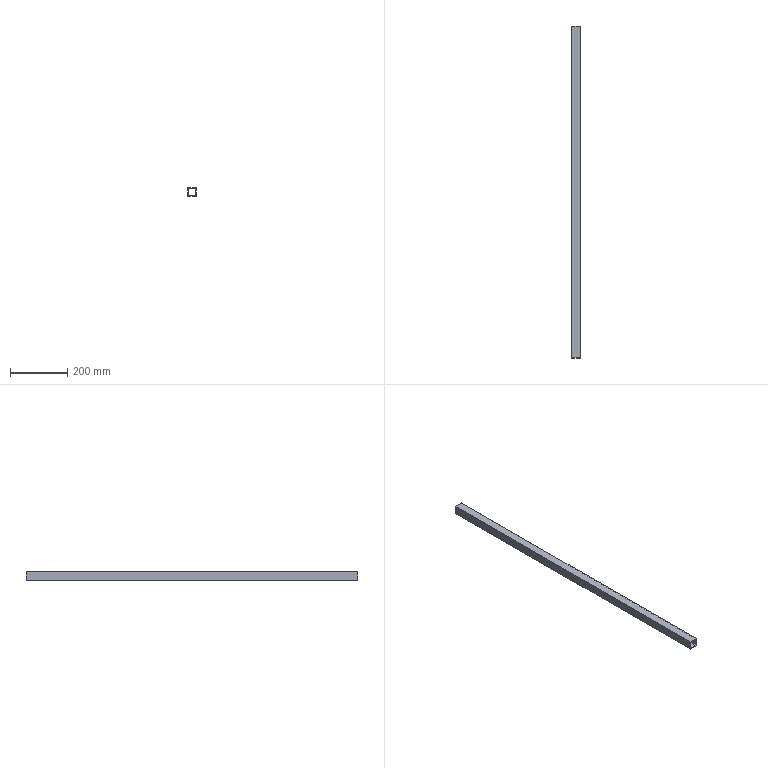Part | NX | features solid 2 | 1 solid | 10 faces | box 30 x 1160 x 30 mm | volume 259840 mm3 | plane 10
STEP:
#1=CARTESIAN_POINT('',(-240.,540.,20.));
#2=VERTEX_POINT('',#1);
#3=CARTESIAN_POINT('',(-210.,540.,20.));
#4=VERTEX_POINT('',#3);
#5=CARTESIAN_POINT('',(-210.,540.,20.));
#6=DIRECTION('',(1.,0.,0.));
#7=VECTOR('',#6,1000.);
#8=LINE('',#5,#7);
#9=EDGE_CURVE('',#2,#4,#8,.T.);
#10=ORIENTED_EDGE('',*,*,#9,.F.);
#11=CARTESIAN_POINT('',(-240.,540.,50.));
#12=VERTEX_POINT('',#11);
#13=CARTESIAN_POINT('',(-240.,540.,50.));
#14=DIRECTION('',(0.,0.,-1.));
#15=VECTOR('',#14,1000.);
#16=LINE('',#13,#15);
#17=EDGE_CURVE('',#12,#2,#16,.T.);
#18=ORIENTED_EDGE('',*,*,#17,.F.);
#19=CARTESIAN_POINT('',(-210.,540.,50.));
#20=VERTEX_POINT('',#19);
#21=CARTESIAN_POINT('',(-210.,540.,50.));
#22=DIRECTION('',(1.,0.,0.));
#23=VECTOR('',#22,1000.);
#24=LINE('',#21,#23);
#25=EDGE_CURVE('',#12,#20,#24,.T.);
#26=ORIENTED_EDGE('',*,*,#25,.T.);
#27=CARTESIAN_POINT('',(-210.,540.,50.));
#28=DIRECTION('',(0.,0.,-1.));
#29=VECTOR('',#28,1000.);
#30=LINE('',#27,#29);
#31=EDGE_CURVE('',#20,#4,#30,.T.);
#32=ORIENTED_EDGE('',*,*,#31,.T.);
#33=EDGE_LOOP('',(#10,#18,#26,#32));
#34=FACE_BOUND('',#33,.T.);
#35=CARTESIAN_POINT('',(-238.,540.,48.));
#36=VERTEX_POINT('',#35);
#37=CARTESIAN_POINT('',(-238.,540.,22.));
#38=VERTEX_POINT('',#37);
#39=CARTESIAN_POINT('',(-238.,540.,50.));
#40=DIRECTION('',(0.,0.,-1.));
#41=VECTOR('',#40,1000.);
#42=LINE('',#39,#41);
#43=EDGE_CURVE('',#36,#38,#42,.T.);
#44=ORIENTED_EDGE('',*,*,#43,.T.);
#45=CARTESIAN_POINT('',(-212.,540.,22.));
#46=VERTEX_POINT('',#45);
#47=CARTESIAN_POINT('',(-210.,540.,22.));
#48=DIRECTION('',(1.,0.,0.));
#49=VECTOR('',#48,1000.);
#50=LINE('',#47,#49);
#51=EDGE_CURVE('',#38,#46,#50,.T.);
#52=ORIENTED_EDGE('',*,*,#51,.T.);
#53=CARTESIAN_POINT('',(-212.,540.,48.));
#54=VERTEX_POINT('',#53);
#55=CARTESIAN_POINT('',(-212.,540.,50.));
#56=DIRECTION('',(0.,0.,-1.));
#57=VECTOR('',#56,1000.);
#58=LINE('',#55,#57);
#59=EDGE_CURVE('',#54,#46,#58,.T.);
#60=ORIENTED_EDGE('',*,*,#59,.F.);
#61=CARTESIAN_POINT('',(-210.,540.,48.));
#62=DIRECTION('',(1.,0.,0.));
#63=VECTOR('',#62,1000.);
#64=LINE('',#61,#63);
#65=EDGE_CURVE('',#36,#54,#64,.T.);
#66=ORIENTED_EDGE('',*,*,#65,.F.);
#67=EDGE_LOOP('',(#44,#52,#60,#66));
#68=FACE_BOUND('',#67,.T.);
#69=CARTESIAN_POINT('',(-240.,540.,50.));
#70=DIRECTION('',(0.,1.,0.));
#71=DIRECTION('',(0.,0.,1.));
#72=AXIS2_PLACEMENT_3D('',#69,#70,#71);
#73=PLANE('',#72);
#74=ADVANCED_FACE('',(#34,#68),#73,.T.);
#75=CARTESIAN_POINT('',(-240.,-620.,20.));
#76=VERTEX_POINT('',#75);
#77=CARTESIAN_POINT('',(-210.,-620.,20.));
#78=VERTEX_POINT('',#77);
#79=CARTESIAN_POINT('',(-210.,-620.,20.));
#80=DIRECTION('',(1.,0.,0.));
#81=VECTOR('',#80,1000.);
#82=LINE('',#79,#81);
#83=EDGE_CURVE('',#76,#78,#82,.T.);
#84=ORIENTED_EDGE('',*,*,#83,.T.);
#85=CARTESIAN_POINT('',(-210.,-620.,50.));
#86=VERTEX_POINT('',#85);
#87=CARTESIAN_POINT('',(-210.,-620.,50.));
#88=DIRECTION('',(0.,0.,-1.));
#89=VECTOR('',#88,1000.);
#90=LINE('',#87,#89);
#91=EDGE_CURVE('',#86,#78,#90,.T.);
#92=ORIENTED_EDGE('',*,*,#91,.F.);
#93=CARTESIAN_POINT('',(-240.,-620.,50.));
#94=VERTEX_POINT('',#93);
#95=CARTESIAN_POINT('',(-210.,-620.,50.));
#96=DIRECTION('',(1.,0.,0.));
#97=VECTOR('',#96,1000.);
#98=LINE('',#95,#97);
#99=EDGE_CURVE('',#94,#86,#98,.T.);
#100=ORIENTED_EDGE('',*,*,#99,.F.);
#101=CARTESIAN_POINT('',(-240.,-620.,50.));
#102=DIRECTION('',(0.,0.,-1.));
#103=VECTOR('',#102,1000.);
#104=LINE('',#101,#103);
#105=EDGE_CURVE('',#94,#76,#104,.T.);
#106=ORIENTED_EDGE('',*,*,#105,.T.);
#107=EDGE_LOOP('',(#84,#92,#100,#106));
#108=FACE_BOUND('',#107,.T.);
#109=CARTESIAN_POINT('',(-238.,-620.,22.));
#110=VERTEX_POINT('',#109);
#111=CARTESIAN_POINT('',(-212.,-620.,22.));
#112=VERTEX_POINT('',#111);
#113=CARTESIAN_POINT('',(-210.,-620.,22.));
#114=DIRECTION('',(1.,0.,0.));
#115=VECTOR('',#114,1000.);
#116=LINE('',#113,#115);
#117=EDGE_CURVE('',#110,#112,#116,.T.);
#118=ORIENTED_EDGE('',*,*,#117,.F.);
#119=CARTESIAN_POINT('',(-238.,-620.,48.));
#120=VERTEX_POINT('',#119);
#121=CARTESIAN_POINT('',(-238.,-620.,50.));
#122=DIRECTION('',(0.,0.,-1.));
#123=VECTOR('',#122,1000.);
#124=LINE('',#121,#123);
#125=EDGE_CURVE('',#120,#110,#124,.T.);
#126=ORIENTED_EDGE('',*,*,#125,.F.);
#127=CARTESIAN_POINT('',(-212.,-620.,48.));
#128=VERTEX_POINT('',#127);
#129=CARTESIAN_POINT('',(-210.,-620.,48.));
#130=DIRECTION('',(1.,0.,0.));
#131=VECTOR('',#130,1000.);
#132=LINE('',#129,#131);
#133=EDGE_CURVE('',#120,#128,#132,.T.);
#134=ORIENTED_EDGE('',*,*,#133,.T.);
#135=CARTESIAN_POINT('',(-212.,-620.,50.));
#136=DIRECTION('',(0.,0.,-1.));
#137=VECTOR('',#136,1000.);
#138=LINE('',#135,#137);
#139=EDGE_CURVE('',#128,#112,#138,.T.);
#140=ORIENTED_EDGE('',*,*,#139,.T.);
#141=EDGE_LOOP('',(#118,#126,#134,#140));
#142=FACE_BOUND('',#141,.T.);
#143=CARTESIAN_POINT('',(-240.,-620.,50.));
#144=DIRECTION('',(0.,1.,0.));
#145=DIRECTION('',(0.,0.,1.));
#146=AXIS2_PLACEMENT_3D('',#143,#144,#145);
#147=PLANE('',#146);
#148=ADVANCED_FACE('',(#108,#142),#147,.F.);
#149=CARTESIAN_POINT('',(-210.,210.,20.));
#150=DIRECTION('',(0.,-1.,0.));
#151=VECTOR('',#150,1000.);
#152=LINE('',#149,#151);
#153=EDGE_CURVE('',#4,#78,#152,.T.);
#154=ORIENTED_EDGE('',*,*,#153,.F.);
#155=ORIENTED_EDGE('',*,*,#31,.F.);
#156=CARTESIAN_POINT('',(-210.,210.,50.));
#157=DIRECTION('',(0.,-1.,0.));
#158=VECTOR('',#157,1000.);
#159=LINE('',#156,#158);
#160=EDGE_CURVE('',#20,#86,#159,.T.);
#161=ORIENTED_EDGE('',*,*,#160,.T.);
#162=ORIENTED_EDGE('',*,*,#91,.T.);
#163=EDGE_LOOP('',(#154,#155,#161,#162));
#164=FACE_BOUND('',#163,.T.);
#165=CARTESIAN_POINT('',(-210.,210.,50.));
#166=DIRECTION('',(1.,0.,0.));
#167=DIRECTION('',(0.,0.,-1.));
#168=AXIS2_PLACEMENT_3D('',#165,#166,#167);
#169=PLANE('',#168);
#170=ADVANCED_FACE('',(#164),#169,.T.);
#171=CARTESIAN_POINT('',(-240.,210.,20.));
#172=DIRECTION('',(0.,-1.,0.));
#173=VECTOR('',#172,1000.);
#174=LINE('',#171,#173);
#175=EDGE_CURVE('',#2,#76,#174,.T.);
#176=ORIENTED_EDGE('',*,*,#175,.T.);
#177=ORIENTED_EDGE('',*,*,#105,.F.);
#178=CARTESIAN_POINT('',(-240.,210.,50.));
#179=DIRECTION('',(0.,-1.,0.));
#180=VECTOR('',#179,1000.);
#181=LINE('',#178,#180);
#182=EDGE_CURVE('',#12,#94,#181,.T.);
#183=ORIENTED_EDGE('',*,*,#182,.F.);
#184=ORIENTED_EDGE('',*,*,#17,.T.);
#185=EDGE_LOOP('',(#176,#177,#183,#184));
#186=FACE_BOUND('',#185,.T.);
#187=CARTESIAN_POINT('',(-240.,210.,50.));
#188=DIRECTION('',(1.,0.,0.));
#189=DIRECTION('',(0.,0.,-1.));
#190=AXIS2_PLACEMENT_3D('',#187,#188,#189);
#191=PLANE('',#190);
#192=ADVANCED_FACE('',(#186),#191,.F.);
#193=ORIENTED_EDGE('',*,*,#25,.F.);
#194=ORIENTED_EDGE('',*,*,#182,.T.);
#195=ORIENTED_EDGE('',*,*,#99,.T.);
#196=ORIENTED_EDGE('',*,*,#160,.F.);
#197=EDGE_LOOP('',(#193,#194,#195,#196));
#198=FACE_BOUND('',#197,.T.);
#199=CARTESIAN_POINT('',(-210.,210.,50.));
#200=DIRECTION('',(0.,0.,-1.));
#201=DIRECTION('',(-1.,0.,0.));
#202=AXIS2_PLACEMENT_3D('',#199,#200,#201);
#203=PLANE('',#202);
#204=ADVANCED_FACE('',(#198),#203,.F.);
#205=ORIENTED_EDGE('',*,*,#9,.T.);
#206=ORIENTED_EDGE('',*,*,#153,.T.);
#207=ORIENTED_EDGE('',*,*,#83,.F.);
#208=ORIENTED_EDGE('',*,*,#175,.F.);
#209=EDGE_LOOP('',(#205,#206,#207,#208));
#210=FACE_BOUND('',#209,.T.);
#211=CARTESIAN_POINT('',(-210.,210.,20.));
#212=DIRECTION('',(0.,0.,-1.));
#213=DIRECTION('',(-1.,0.,0.));
#214=AXIS2_PLACEMENT_3D('',#211,#212,#213);
#215=PLANE('',#214);
#216=ADVANCED_FACE('',(#210),#215,.T.);
#217=CARTESIAN_POINT('',(-212.,210.,22.));
#218=DIRECTION('',(0.,-1.,0.));
#219=VECTOR('',#218,1000.);
#220=LINE('',#217,#219);
#221=EDGE_CURVE('',#46,#112,#220,.T.);
#222=ORIENTED_EDGE('',*,*,#221,.T.);
#223=ORIENTED_EDGE('',*,*,#139,.F.);
#224=CARTESIAN_POINT('',(-212.,210.,48.));
#225=DIRECTION('',(0.,-1.,0.));
#226=VECTOR('',#225,1000.);
#227=LINE('',#224,#226);
#228=EDGE_CURVE('',#54,#128,#227,.T.);
#229=ORIENTED_EDGE('',*,*,#228,.F.);
#230=ORIENTED_EDGE('',*,*,#59,.T.);
#231=EDGE_LOOP('',(#222,#223,#229,#230));
#232=FACE_BOUND('',#231,.T.);
#233=CARTESIAN_POINT('',(-212.,210.,50.));
#234=DIRECTION('',(1.,0.,0.));
#235=DIRECTION('',(0.,0.,-1.));
#236=AXIS2_PLACEMENT_3D('',#233,#234,#235);
#237=PLANE('',#236);
#238=ADVANCED_FACE('',(#232),#237,.F.);
#239=CARTESIAN_POINT('',(-238.,210.,22.));
#240=DIRECTION('',(0.,-1.,0.));
#241=VECTOR('',#240,1000.);
#242=LINE('',#239,#241);
#243=EDGE_CURVE('',#38,#110,#242,.T.);
#244=ORIENTED_EDGE('',*,*,#243,.F.);
#245=ORIENTED_EDGE('',*,*,#43,.F.);
#246=CARTESIAN_POINT('',(-238.,210.,48.));
#247=DIRECTION('',(0.,-1.,0.));
#248=VECTOR('',#247,1000.);
#249=LINE('',#246,#248);
#250=EDGE_CURVE('',#36,#120,#249,.T.);
#251=ORIENTED_EDGE('',*,*,#250,.T.);
#252=ORIENTED_EDGE('',*,*,#125,.T.);
#253=EDGE_LOOP('',(#244,#245,#251,#252));
#254=FACE_BOUND('',#253,.T.);
#255=CARTESIAN_POINT('',(-238.,210.,50.));
#256=DIRECTION('',(1.,0.,0.));
#257=DIRECTION('',(0.,0.,-1.));
#258=AXIS2_PLACEMENT_3D('',#255,#256,#257);
#259=PLANE('',#258);
#260=ADVANCED_FACE('',(#254),#259,.T.);
#261=ORIENTED_EDGE('',*,*,#65,.T.);
#262=ORIENTED_EDGE('',*,*,#228,.T.);
#263=ORIENTED_EDGE('',*,*,#133,.F.);
#264=ORIENTED_EDGE('',*,*,#250,.F.);
#265=EDGE_LOOP('',(#261,#262,#263,#264));
#266=FACE_BOUND('',#265,.T.);
#267=CARTESIAN_POINT('',(-210.,210.,48.));
#268=DIRECTION('',(0.,0.,-1.));
#269=DIRECTION('',(-1.,0.,0.));
#270=AXIS2_PLACEMENT_3D('',#267,#268,#269);
#271=PLANE('',#270);
#272=ADVANCED_FACE('',(#266),#271,.T.);
#273=ORIENTED_EDGE('',*,*,#51,.F.);
#274=ORIENTED_EDGE('',*,*,#243,.T.);
#275=ORIENTED_EDGE('',*,*,#117,.T.);
#276=ORIENTED_EDGE('',*,*,#221,.F.);
#277=EDGE_LOOP('',(#273,#274,#275,#276));
#278=FACE_BOUND('',#277,.T.);
#279=CARTESIAN_POINT('',(-210.,210.,22.));
#280=DIRECTION('',(0.,0.,-1.));
#281=DIRECTION('',(-1.,0.,0.));
#282=AXIS2_PLACEMENT_3D('',#279,#280,#281);
#283=PLANE('',#282);
#284=ADVANCED_FACE('',(#278),#283,.F.);
#285=CLOSED_SHELL('',(#74,#148,#170,#192,#204,#216,#238,#260,#272,#284));
#286=MANIFOLD_SOLID_BREP('',#285);
#287=(LENGTH_UNIT()NAMED_UNIT(*)SI_UNIT(.MILLI.,.METRE.));
#288=UNCERTAINTY_MEASURE_WITH_UNIT(LENGTH_MEASURE(0.00001),#287,'','');
#289=(NAMED_UNIT(*)PLANE_ANGLE_UNIT()SI_UNIT($,.RADIAN.));
#290=(NAMED_UNIT(*)SI_UNIT($,.STERADIAN.)SOLID_ANGLE_UNIT());
#291=(GEOMETRIC_REPRESENTATION_CONTEXT(3)GLOBAL_UNCERTAINTY_ASSIGNED_CONTEXT((#288))GLOBAL_UNIT_ASSIGNED_CONTEXT((#287,#289,#290))REPRESENTATION_CONTEXT('',''));
#292=ADVANCED_BREP_SHAPE_REPRESENTATION('',(#286),#291);